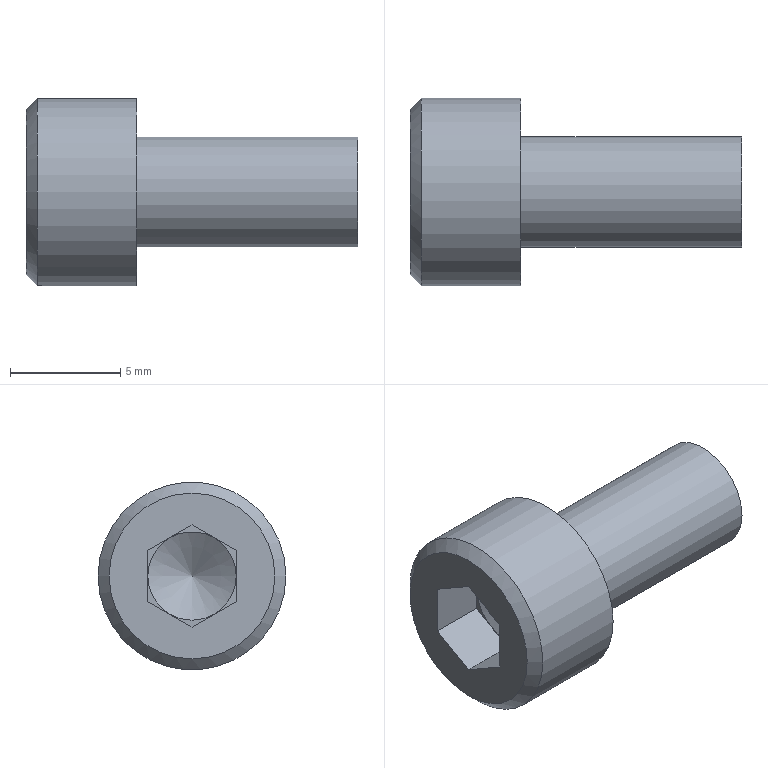Part | NX | features 5003_320_CB5-10 2 | 1 solid | 19 faces | box 15 x 8.5 x 8.5 mm | volume 437.193 mm3 | plane 15 | cylinder 2 | cone 2 | commonest cylinder face diameters 5 x1 8.5 x1
STEP:
#1=CARTESIAN_POINT('',(178.225,-20.25,-12.5));
#2=VERTEX_POINT('',#1);
#3=CARTESIAN_POINT('',(178.225,-24.,-12.5));
#4=DIRECTION('',(1.,0.,0.));
#5=DIRECTION('',(0.,1.,0.));
#6=AXIS2_PLACEMENT_3D('',#3,#4,#5);
#7=CIRCLE('',#6,3.75);
#8=EDGE_CURVE('',#2,#2,#7,.F.);
#9=ORIENTED_EDGE('',*,*,#8,.T.);
#10=EDGE_LOOP('',(#9));
#11=FACE_BOUND('',#10,.T.);
#12=CARTESIAN_POINT('',(178.225,-24.,-14.809));
#13=VERTEX_POINT('',#12);
#14=CARTESIAN_POINT('',(178.225,-26.,-13.655));
#15=VERTEX_POINT('',#14);
#16=CARTESIAN_POINT('',(178.225,-24.,-14.809));
#17=DIRECTION('',(0.,-0.866,0.5));
#18=VECTOR('',#17,1000.);
#19=LINE('',#16,#18);
#20=EDGE_CURVE('',#13,#15,#19,.T.);
#21=ORIENTED_EDGE('',*,*,#20,.F.);
#22=CARTESIAN_POINT('',(178.225,-22.,-13.655));
#23=VERTEX_POINT('',#22);
#24=CARTESIAN_POINT('',(178.225,-22.,-13.655));
#25=DIRECTION('',(0.,-0.866,-0.5));
#26=VECTOR('',#25,1000.);
#27=LINE('',#24,#26);
#28=EDGE_CURVE('',#23,#13,#27,.T.);
#29=ORIENTED_EDGE('',*,*,#28,.F.);
#30=CARTESIAN_POINT('',(178.225,-22.,-11.345));
#31=VERTEX_POINT('',#30);
#32=CARTESIAN_POINT('',(178.225,-22.,-11.345));
#33=DIRECTION('',(0.,0.,-1.));
#34=VECTOR('',#33,1000.);
#35=LINE('',#32,#34);
#36=EDGE_CURVE('',#31,#23,#35,.T.);
#37=ORIENTED_EDGE('',*,*,#36,.F.);
#38=CARTESIAN_POINT('',(178.225,-24.,-10.191));
#39=VERTEX_POINT('',#38);
#40=CARTESIAN_POINT('',(178.225,-24.,-10.191));
#41=DIRECTION('',(0.,0.866,-0.5));
#42=VECTOR('',#41,1000.);
#43=LINE('',#40,#42);
#44=EDGE_CURVE('',#39,#31,#43,.T.);
#45=ORIENTED_EDGE('',*,*,#44,.F.);
#46=CARTESIAN_POINT('',(178.225,-26.,-11.345));
#47=VERTEX_POINT('',#46);
#48=CARTESIAN_POINT('',(178.225,-26.,-11.345));
#49=DIRECTION('',(0.,0.866,0.5));
#50=VECTOR('',#49,1000.);
#51=LINE('',#48,#50);
#52=EDGE_CURVE('',#47,#39,#51,.T.);
#53=ORIENTED_EDGE('',*,*,#52,.F.);
#54=CARTESIAN_POINT('',(178.225,-26.,-13.655));
#55=DIRECTION('',(0.,0.,1.));
#56=VECTOR('',#55,1000.);
#57=LINE('',#54,#56);
#58=EDGE_CURVE('',#15,#47,#57,.T.);
#59=ORIENTED_EDGE('',*,*,#58,.F.);
#60=EDGE_LOOP('',(#21,#29,#37,#45,#53,#59));
#61=FACE_BOUND('',#60,.T.);
#62=CARTESIAN_POINT('',(178.225,-24.,-8.25));
#63=DIRECTION('',(1.,0.,0.));
#64=DIRECTION('',(0.,1.,0.));
#65=AXIS2_PLACEMENT_3D('',#62,#63,#64);
#66=PLANE('',#65);
#67=ADVANCED_FACE('',(#11,#61),#66,.F.);
#68=CARTESIAN_POINT('',(193.225,-26.5,-12.5));
#69=VERTEX_POINT('',#68);
#70=CARTESIAN_POINT('',(193.225,-24.,-12.5));
#71=DIRECTION('',(-1.,0.,0.));
#72=DIRECTION('',(0.,-1.,0.));
#73=AXIS2_PLACEMENT_3D('',#70,#71,#72);
#74=CIRCLE('',#73,2.5);
#75=EDGE_CURVE('',#69,#69,#74,.T.);
#76=ORIENTED_EDGE('',*,*,#75,.F.);
#77=EDGE_LOOP('',(#76));
#78=FACE_BOUND('',#77,.T.);
#79=CARTESIAN_POINT('',(193.225,-24.,-12.5));
#80=DIRECTION('',(-1.,0.,0.));
#81=DIRECTION('',(0.,-1.,0.));
#82=AXIS2_PLACEMENT_3D('',#79,#80,#81);
#83=PLANE('',#82);
#84=ADVANCED_FACE('',(#78),#83,.F.);
#85=CARTESIAN_POINT('',(183.225,-26.5,-12.5));
#86=VERTEX_POINT('',#85);
#87=CARTESIAN_POINT('',(183.225,-24.,-12.5));
#88=DIRECTION('',(-1.,0.,0.));
#89=DIRECTION('',(0.,-1.,0.));
#90=AXIS2_PLACEMENT_3D('',#87,#88,#89);
#91=CIRCLE('',#90,2.5);
#92=EDGE_CURVE('',#86,#86,#91,.T.);
#93=ORIENTED_EDGE('',*,*,#92,.F.);
#94=EDGE_LOOP('',(#93));
#95=FACE_BOUND('',#94,.T.);
#96=ORIENTED_EDGE('',*,*,#75,.T.);
#97=EDGE_LOOP('',(#96));
#98=FACE_BOUND('',#97,.T.);
#99=CARTESIAN_POINT('',(178.225,-24.,-12.5));
#100=DIRECTION('',(-1.,0.,0.));
#101=DIRECTION('',(0.,-1.,0.));
#102=AXIS2_PLACEMENT_3D('',#99,#100,#101);
#103=CYLINDRICAL_SURFACE('',#102,2.5);
#104=ADVANCED_FACE('',(#95,#98),#103,.T.);
#105=CARTESIAN_POINT('',(183.225,-28.25,-12.5));
#106=VERTEX_POINT('',#105);
#107=CARTESIAN_POINT('',(183.225,-24.,-12.5));
#108=DIRECTION('',(-1.,0.,0.));
#109=DIRECTION('',(0.,-1.,0.));
#110=AXIS2_PLACEMENT_3D('',#107,#108,#109);
#111=CIRCLE('',#110,4.25);
#112=EDGE_CURVE('',#106,#106,#111,.T.);
#113=ORIENTED_EDGE('',*,*,#112,.F.);
#114=EDGE_LOOP('',(#113));
#115=FACE_BOUND('',#114,.T.);
#116=ORIENTED_EDGE('',*,*,#92,.T.);
#117=EDGE_LOOP('',(#116));
#118=FACE_BOUND('',#117,.T.);
#119=CARTESIAN_POINT('',(183.225,-24.,-10.));
#120=DIRECTION('',(-1.,0.,0.));
#121=DIRECTION('',(0.,-1.,0.));
#122=AXIS2_PLACEMENT_3D('',#119,#120,#121);
#123=PLANE('',#122);
#124=ADVANCED_FACE('',(#115,#118),#123,.F.);
#125=CARTESIAN_POINT('',(178.725,-19.75,-12.5));
#126=VERTEX_POINT('',#125);
#127=CARTESIAN_POINT('',(178.725,-24.,-12.5));
#128=DIRECTION('',(1.,0.,0.));
#129=DIRECTION('',(0.,1.,0.));
#130=AXIS2_PLACEMENT_3D('',#127,#128,#129);
#131=CIRCLE('',#130,4.25);
#132=EDGE_CURVE('',#126,#126,#131,.T.);
#133=ORIENTED_EDGE('',*,*,#132,.T.);
#134=EDGE_LOOP('',(#133));
#135=FACE_BOUND('',#134,.T.);
#136=ORIENTED_EDGE('',*,*,#112,.T.);
#137=EDGE_LOOP('',(#136));
#138=FACE_BOUND('',#137,.T.);
#139=CARTESIAN_POINT('',(178.225,-24.,-12.5));
#140=DIRECTION('',(-1.,0.,0.));
#141=DIRECTION('',(0.,-1.,0.));
#142=AXIS2_PLACEMENT_3D('',#139,#140,#141);
#143=CYLINDRICAL_SURFACE('',#142,4.25);
#144=ADVANCED_FACE('',(#135,#138),#143,.T.);
#145=ORIENTED_EDGE('',*,*,#132,.F.);
#146=EDGE_LOOP('',(#145));
#147=FACE_BOUND('',#146,.T.);
#148=ORIENTED_EDGE('',*,*,#8,.F.);
#149=EDGE_LOOP('',(#148));
#150=FACE_BOUND('',#149,.T.);
#151=CARTESIAN_POINT('',(178.225,-24.,-12.5));
#152=DIRECTION('',(1.,0.,0.));
#153=DIRECTION('',(0.,1.,0.));
#154=AXIS2_PLACEMENT_3D('',#151,#152,#153);
#155=CONICAL_SURFACE('',#154,3.75,0.7854);
#156=ADVANCED_FACE('',(#147,#150),#155,.T.);
#157=CARTESIAN_POINT('',(180.725,-22.,-13.655));
#158=VERTEX_POINT('',#157);
#159=CARTESIAN_POINT('',(180.725,-23.,-14.232));
#160=VERTEX_POINT('',#159);
#161=CARTESIAN_POINT('',(180.725,-22.,-13.655));
#162=DIRECTION('',(0.,-0.866,-0.5));
#163=VECTOR('',#162,1000.);
#164=LINE('',#161,#163);
#165=EDGE_CURVE('',#158,#160,#164,.T.);
#166=ORIENTED_EDGE('',*,*,#165,.F.);
#167=CARTESIAN_POINT('',(180.725,-22.,-13.655));
#168=DIRECTION('',(-1.,0.,0.));
#169=VECTOR('',#168,1000.);
#170=LINE('',#167,#169);
#171=EDGE_CURVE('',#158,#23,#170,.T.);
#172=ORIENTED_EDGE('',*,*,#171,.T.);
#173=ORIENTED_EDGE('',*,*,#28,.T.);
#174=CARTESIAN_POINT('',(180.725,-24.,-14.809));
#175=VERTEX_POINT('',#174);
#176=CARTESIAN_POINT('',(180.725,-24.,-14.809));
#177=DIRECTION('',(-1.,0.,0.));
#178=VECTOR('',#177,1000.);
#179=LINE('',#176,#178);
#180=EDGE_CURVE('',#175,#13,#179,.T.);
#181=ORIENTED_EDGE('',*,*,#180,.F.);
#182=CARTESIAN_POINT('',(180.725,-22.,-13.655));
#183=DIRECTION('',(0.,-0.866,-0.5));
#184=VECTOR('',#183,1000.);
#185=LINE('',#182,#184);
#186=EDGE_CURVE('',#160,#175,#185,.T.);
#187=ORIENTED_EDGE('',*,*,#186,.F.);
#188=EDGE_LOOP('',(#166,#172,#173,#181,#187));
#189=FACE_BOUND('',#188,.T.);
#190=CARTESIAN_POINT('',(180.725,-22.,-13.655));
#191=DIRECTION('',(0.,0.5,-0.866));
#192=DIRECTION('',(0.,0.866,0.5));
#193=AXIS2_PLACEMENT_3D('',#190,#191,#192);
#194=PLANE('',#193);
#195=ADVANCED_FACE('',(#189),#194,.F.);
#196=CARTESIAN_POINT('',(180.725,-22.,-11.345));
#197=VERTEX_POINT('',#196);
#198=CARTESIAN_POINT('',(180.725,-22.,-12.5));
#199=VERTEX_POINT('',#198);
#200=CARTESIAN_POINT('',(180.725,-22.,-11.345));
#201=DIRECTION('',(0.,0.,-1.));
#202=VECTOR('',#201,1000.);
#203=LINE('',#200,#202);
#204=EDGE_CURVE('',#197,#199,#203,.T.);
#205=ORIENTED_EDGE('',*,*,#204,.F.);
#206=CARTESIAN_POINT('',(180.725,-22.,-11.345));
#207=DIRECTION('',(-1.,0.,0.));
#208=VECTOR('',#207,1000.);
#209=LINE('',#206,#208);
#210=EDGE_CURVE('',#197,#31,#209,.T.);
#211=ORIENTED_EDGE('',*,*,#210,.T.);
#212=ORIENTED_EDGE('',*,*,#36,.T.);
#213=ORIENTED_EDGE('',*,*,#171,.F.);
#214=CARTESIAN_POINT('',(180.725,-22.,-11.345));
#215=DIRECTION('',(0.,0.,-1.));
#216=VECTOR('',#215,1000.);
#217=LINE('',#214,#216);
#218=EDGE_CURVE('',#199,#158,#217,.T.);
#219=ORIENTED_EDGE('',*,*,#218,.F.);
#220=EDGE_LOOP('',(#205,#211,#212,#213,#219));
#221=FACE_BOUND('',#220,.T.);
#222=CARTESIAN_POINT('',(180.725,-22.,-11.345));
#223=DIRECTION('',(0.,1.,0.));
#224=DIRECTION('',(-1.,0.,0.));
#225=AXIS2_PLACEMENT_3D('',#222,#223,#224);
#226=PLANE('',#225);
#227=ADVANCED_FACE('',(#221),#226,.F.);
#228=CARTESIAN_POINT('',(180.725,-24.,-10.191));
#229=VERTEX_POINT('',#228);
#230=CARTESIAN_POINT('',(180.725,-23.,-10.768));
#231=VERTEX_POINT('',#230);
#232=CARTESIAN_POINT('',(180.725,-24.,-10.191));
#233=DIRECTION('',(0.,0.866,-0.5));
#234=VECTOR('',#233,1000.);
#235=LINE('',#232,#234);
#236=EDGE_CURVE('',#229,#231,#235,.T.);
#237=ORIENTED_EDGE('',*,*,#236,.F.);
#238=CARTESIAN_POINT('',(180.725,-24.,-10.191));
#239=DIRECTION('',(-1.,0.,0.));
#240=VECTOR('',#239,1000.);
#241=LINE('',#238,#240);
#242=EDGE_CURVE('',#229,#39,#241,.T.);
#243=ORIENTED_EDGE('',*,*,#242,.T.);
#244=ORIENTED_EDGE('',*,*,#44,.T.);
#245=ORIENTED_EDGE('',*,*,#210,.F.);
#246=CARTESIAN_POINT('',(180.725,-24.,-10.191));
#247=DIRECTION('',(0.,0.866,-0.5));
#248=VECTOR('',#247,1000.);
#249=LINE('',#246,#248);
#250=EDGE_CURVE('',#231,#197,#249,.T.);
#251=ORIENTED_EDGE('',*,*,#250,.F.);
#252=EDGE_LOOP('',(#237,#243,#244,#245,#251));
#253=FACE_BOUND('',#252,.T.);
#254=CARTESIAN_POINT('',(180.725,-24.,-10.191));
#255=DIRECTION('',(0.,0.5,0.866));
#256=DIRECTION('',(0.,-0.866,0.5));
#257=AXIS2_PLACEMENT_3D('',#254,#255,#256);
#258=PLANE('',#257);
#259=ADVANCED_FACE('',(#253),#258,.F.);
#260=CARTESIAN_POINT('',(180.725,-26.,-11.345));
#261=VERTEX_POINT('',#260);
#262=CARTESIAN_POINT('',(180.725,-25.,-10.768));
#263=VERTEX_POINT('',#262);
#264=CARTESIAN_POINT('',(180.725,-26.,-11.345));
#265=DIRECTION('',(0.,0.866,0.5));
#266=VECTOR('',#265,1000.);
#267=LINE('',#264,#266);
#268=EDGE_CURVE('',#261,#263,#267,.T.);
#269=ORIENTED_EDGE('',*,*,#268,.F.);
#270=CARTESIAN_POINT('',(180.725,-26.,-11.345));
#271=DIRECTION('',(-1.,0.,0.));
#272=VECTOR('',#271,1000.);
#273=LINE('',#270,#272);
#274=EDGE_CURVE('',#261,#47,#273,.T.);
#275=ORIENTED_EDGE('',*,*,#274,.T.);
#276=ORIENTED_EDGE('',*,*,#52,.T.);
#277=ORIENTED_EDGE('',*,*,#242,.F.);
#278=CARTESIAN_POINT('',(180.725,-26.,-11.345));
#279=DIRECTION('',(0.,0.866,0.5));
#280=VECTOR('',#279,1000.);
#281=LINE('',#278,#280);
#282=EDGE_CURVE('',#263,#229,#281,.T.);
#283=ORIENTED_EDGE('',*,*,#282,.F.);
#284=EDGE_LOOP('',(#269,#275,#276,#277,#283));
#285=FACE_BOUND('',#284,.T.);
#286=CARTESIAN_POINT('',(180.725,-26.,-11.345));
#287=DIRECTION('',(0.,-0.5,0.866));
#288=DIRECTION('',(0.,-0.866,-0.5));
#289=AXIS2_PLACEMENT_3D('',#286,#287,#288);
#290=PLANE('',#289);
#291=ADVANCED_FACE('',(#285),#290,.F.);
#292=CARTESIAN_POINT('',(180.725,-26.,-13.655));
#293=VERTEX_POINT('',#292);
#294=CARTESIAN_POINT('',(180.725,-26.,-12.5));
#295=VERTEX_POINT('',#294);
#296=CARTESIAN_POINT('',(180.725,-26.,-13.655));
#297=DIRECTION('',(0.,0.,1.));
#298=VECTOR('',#297,1000.);
#299=LINE('',#296,#298);
#300=EDGE_CURVE('',#293,#295,#299,.T.);
#301=ORIENTED_EDGE('',*,*,#300,.F.);
#302=CARTESIAN_POINT('',(180.725,-26.,-13.655));
#303=DIRECTION('',(-1.,0.,0.));
#304=VECTOR('',#303,1000.);
#305=LINE('',#302,#304);
#306=EDGE_CURVE('',#293,#15,#305,.T.);
#307=ORIENTED_EDGE('',*,*,#306,.T.);
#308=ORIENTED_EDGE('',*,*,#58,.T.);
#309=ORIENTED_EDGE('',*,*,#274,.F.);
#310=CARTESIAN_POINT('',(180.725,-26.,-13.655));
#311=DIRECTION('',(0.,0.,1.));
#312=VECTOR('',#311,1000.);
#313=LINE('',#310,#312);
#314=EDGE_CURVE('',#295,#261,#313,.T.);
#315=ORIENTED_EDGE('',*,*,#314,.F.);
#316=EDGE_LOOP('',(#301,#307,#308,#309,#315));
#317=FACE_BOUND('',#316,.T.);
#318=CARTESIAN_POINT('',(180.725,-26.,-13.655));
#319=DIRECTION('',(0.,-1.,0.));
#320=DIRECTION('',(0.,0.,-1.));
#321=AXIS2_PLACEMENT_3D('',#318,#319,#320);
#322=PLANE('',#321);
#323=ADVANCED_FACE('',(#317),#322,.F.);
#324=CARTESIAN_POINT('',(180.725,-25.,-14.232));
#325=VERTEX_POINT('',#324);
#326=CARTESIAN_POINT('',(180.725,-24.,-14.809));
#327=DIRECTION('',(0.,-0.866,0.5));
#328=VECTOR('',#327,1000.);
#329=LINE('',#326,#328);
#330=EDGE_CURVE('',#175,#325,#329,.T.);
#331=ORIENTED_EDGE('',*,*,#330,.F.);
#332=ORIENTED_EDGE('',*,*,#180,.T.);
#333=ORIENTED_EDGE('',*,*,#20,.T.);
#334=ORIENTED_EDGE('',*,*,#306,.F.);
#335=CARTESIAN_POINT('',(180.725,-24.,-14.809));
#336=DIRECTION('',(0.,-0.866,0.5));
#337=VECTOR('',#336,1000.);
#338=LINE('',#335,#337);
#339=EDGE_CURVE('',#325,#293,#338,.T.);
#340=ORIENTED_EDGE('',*,*,#339,.F.);
#341=EDGE_LOOP('',(#331,#332,#333,#334,#340));
#342=FACE_BOUND('',#341,.T.);
#343=CARTESIAN_POINT('',(180.725,-24.,-14.809));
#344=DIRECTION('',(0.,-0.5,-0.866));
#345=DIRECTION('',(0.,0.866,-0.5));
#346=AXIS2_PLACEMENT_3D('',#343,#344,#345);
#347=PLANE('',#346);
#348=ADVANCED_FACE('',(#342),#347,.F.);
#349=ORIENTED_EDGE('',*,*,#314,.T.);
#350=ORIENTED_EDGE('',*,*,#268,.T.);
#351=CARTESIAN_POINT('',(180.725,-24.,-12.5));
#352=DIRECTION('',(-1.,0.,0.));
#353=DIRECTION('',(0.,0.,-1.));
#354=AXIS2_PLACEMENT_3D('',#351,#352,#353);
#355=CIRCLE('',#354,2.);
#356=EDGE_CURVE('',#295,#263,#355,.T.);
#357=ORIENTED_EDGE('',*,*,#356,.F.);
#358=EDGE_LOOP('',(#349,#350,#357));
#359=FACE_BOUND('',#358,.T.);
#360=CARTESIAN_POINT('',(180.725,-24.,-12.5));
#361=DIRECTION('',(-1.,0.,0.));
#362=DIRECTION('',(0.,-1.,0.));
#363=AXIS2_PLACEMENT_3D('',#360,#361,#362);
#364=PLANE('',#363);
#365=ADVANCED_FACE('',(#359),#364,.T.);
#366=ORIENTED_EDGE('',*,*,#282,.T.);
#367=ORIENTED_EDGE('',*,*,#236,.T.);
#368=CARTESIAN_POINT('',(180.725,-24.,-12.5));
#369=DIRECTION('',(-1.,0.,0.));
#370=DIRECTION('',(0.,0.,-1.));
#371=AXIS2_PLACEMENT_3D('',#368,#369,#370);
#372=CIRCLE('',#371,2.);
#373=EDGE_CURVE('',#263,#231,#372,.T.);
#374=ORIENTED_EDGE('',*,*,#373,.F.);
#375=EDGE_LOOP('',(#366,#367,#374));
#376=FACE_BOUND('',#375,.T.);
#377=CARTESIAN_POINT('',(180.725,-24.,-12.5));
#378=DIRECTION('',(-1.,0.,0.));
#379=DIRECTION('',(0.,-1.,0.));
#380=AXIS2_PLACEMENT_3D('',#377,#378,#379);
#381=PLANE('',#380);
#382=ADVANCED_FACE('',(#376),#381,.T.);
#383=ORIENTED_EDGE('',*,*,#250,.T.);
#384=ORIENTED_EDGE('',*,*,#204,.T.);
#385=CARTESIAN_POINT('',(180.725,-24.,-12.5));
#386=DIRECTION('',(-1.,0.,0.));
#387=DIRECTION('',(0.,0.,-1.));
#388=AXIS2_PLACEMENT_3D('',#385,#386,#387);
#389=CIRCLE('',#388,2.);
#390=EDGE_CURVE('',#231,#199,#389,.T.);
#391=ORIENTED_EDGE('',*,*,#390,.F.);
#392=EDGE_LOOP('',(#383,#384,#391));
#393=FACE_BOUND('',#392,.T.);
#394=CARTESIAN_POINT('',(180.725,-24.,-12.5));
#395=DIRECTION('',(-1.,0.,0.));
#396=DIRECTION('',(0.,-1.,0.));
#397=AXIS2_PLACEMENT_3D('',#394,#395,#396);
#398=PLANE('',#397);
#399=ADVANCED_FACE('',(#393),#398,.T.);
#400=ORIENTED_EDGE('',*,*,#218,.T.);
#401=ORIENTED_EDGE('',*,*,#165,.T.);
#402=CARTESIAN_POINT('',(180.725,-24.,-12.5));
#403=DIRECTION('',(-1.,0.,0.));
#404=DIRECTION('',(0.,0.,-1.));
#405=AXIS2_PLACEMENT_3D('',#402,#403,#404);
#406=CIRCLE('',#405,2.);
#407=EDGE_CURVE('',#199,#160,#406,.T.);
#408=ORIENTED_EDGE('',*,*,#407,.F.);
#409=EDGE_LOOP('',(#400,#401,#408));
#410=FACE_BOUND('',#409,.T.);
#411=CARTESIAN_POINT('',(180.725,-24.,-12.5));
#412=DIRECTION('',(-1.,0.,0.));
#413=DIRECTION('',(0.,-1.,0.));
#414=AXIS2_PLACEMENT_3D('',#411,#412,#413);
#415=PLANE('',#414);
#416=ADVANCED_FACE('',(#410),#415,.T.);
#417=ORIENTED_EDGE('',*,*,#186,.T.);
#418=ORIENTED_EDGE('',*,*,#330,.T.);
#419=CARTESIAN_POINT('',(180.725,-24.,-12.5));
#420=DIRECTION('',(-1.,0.,0.));
#421=DIRECTION('',(0.,0.,-1.));
#422=AXIS2_PLACEMENT_3D('',#419,#420,#421);
#423=CIRCLE('',#422,2.);
#424=EDGE_CURVE('',#160,#325,#423,.T.);
#425=ORIENTED_EDGE('',*,*,#424,.F.);
#426=EDGE_LOOP('',(#417,#418,#425));
#427=FACE_BOUND('',#426,.T.);
#428=CARTESIAN_POINT('',(180.725,-24.,-12.5));
#429=DIRECTION('',(-1.,0.,0.));
#430=DIRECTION('',(0.,-1.,0.));
#431=AXIS2_PLACEMENT_3D('',#428,#429,#430);
#432=PLANE('',#431);
#433=ADVANCED_FACE('',(#427),#432,.T.);
#434=ORIENTED_EDGE('',*,*,#339,.T.);
#435=ORIENTED_EDGE('',*,*,#300,.T.);
#436=CARTESIAN_POINT('',(180.725,-24.,-12.5));
#437=DIRECTION('',(-1.,0.,0.));
#438=DIRECTION('',(0.,0.,-1.));
#439=AXIS2_PLACEMENT_3D('',#436,#437,#438);
#440=CIRCLE('',#439,2.);
#441=EDGE_CURVE('',#325,#295,#440,.T.);
#442=ORIENTED_EDGE('',*,*,#441,.F.);
#443=EDGE_LOOP('',(#434,#435,#442));
#444=FACE_BOUND('',#443,.T.);
#445=CARTESIAN_POINT('',(180.725,-24.,-12.5));
#446=DIRECTION('',(-1.,0.,0.));
#447=DIRECTION('',(0.,-1.,0.));
#448=AXIS2_PLACEMENT_3D('',#445,#446,#447);
#449=PLANE('',#448);
#450=ADVANCED_FACE('',(#444),#449,.T.);
#451=ORIENTED_EDGE('',*,*,#441,.T.);
#452=ORIENTED_EDGE('',*,*,#356,.T.);
#453=ORIENTED_EDGE('',*,*,#373,.T.);
#454=ORIENTED_EDGE('',*,*,#390,.T.);
#455=ORIENTED_EDGE('',*,*,#407,.T.);
#456=ORIENTED_EDGE('',*,*,#424,.T.);
#457=EDGE_LOOP('',(#451,#452,#453,#454,#455,#456));
#458=FACE_BOUND('',#457,.T.);
#459=CARTESIAN_POINT('',(181.927,-24.,-12.5));
#460=VERTEX_POINT('',#459);
#461=VERTEX_LOOP('',#460);
#462=FACE_BOUND('',#461,.T.);
#463=CARTESIAN_POINT('',(181.927,-24.,-12.5));
#464=DIRECTION('',(-1.,0.,0.));
#465=DIRECTION('',(0.,0.,-1.));
#466=AXIS2_PLACEMENT_3D('',#463,#464,#465);
#467=CONICAL_SURFACE('',#466,0.,1.03);
#468=ADVANCED_FACE('',(#458,#462),#467,.F.);
#469=CLOSED_SHELL('',(#67,#84,#104,#124,#144,#156,#195,#227,#259,#291,#323,#348,#365,#382,#399,#416,#433,#450,#468));
#470=MANIFOLD_SOLID_BREP('',#469);
#471=(LENGTH_UNIT()NAMED_UNIT(*)SI_UNIT(.MILLI.,.METRE.));
#472=UNCERTAINTY_MEASURE_WITH_UNIT(LENGTH_MEASURE(0.00001),#471,'','');
#473=(NAMED_UNIT(*)PLANE_ANGLE_UNIT()SI_UNIT($,.RADIAN.));
#474=(NAMED_UNIT(*)SI_UNIT($,.STERADIAN.)SOLID_ANGLE_UNIT());
#475=(GEOMETRIC_REPRESENTATION_CONTEXT(3)GLOBAL_UNCERTAINTY_ASSIGNED_CONTEXT((#472))GLOBAL_UNIT_ASSIGNED_CONTEXT((#471,#473,#474))REPRESENTATION_CONTEXT('',''));
#476=ADVANCED_BREP_SHAPE_REPRESENTATION('',(#470),#475);